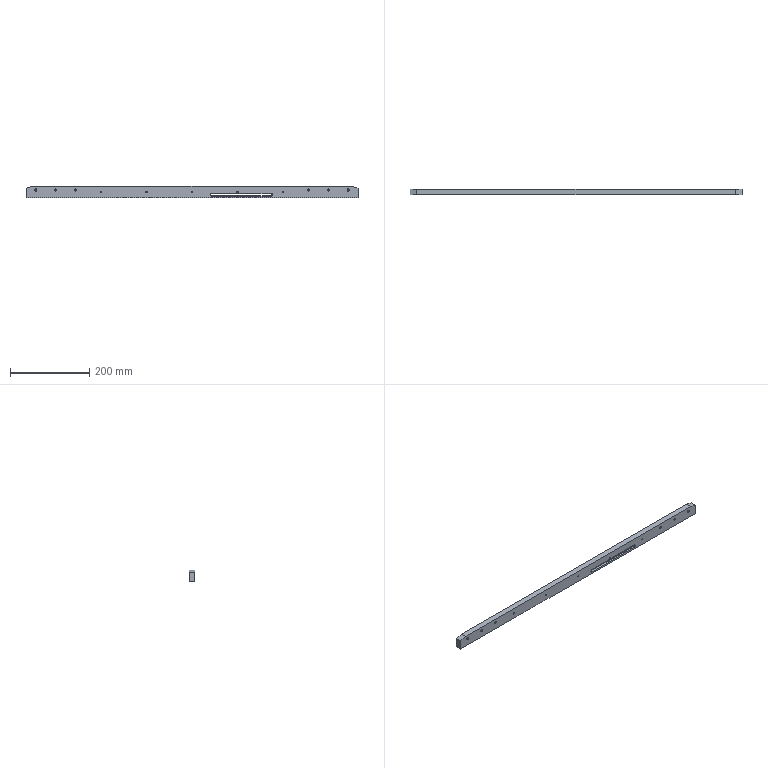Part | STEP file | Rail | 1 solid | 67 faces | box 840 x 15 x 30 mm | volume 357627 mm3 | cylinder 38 | plane 19 | cone 10 | commonest cylinder face diameters 5.5 x14 10 x12 3.3 x10 8 x2